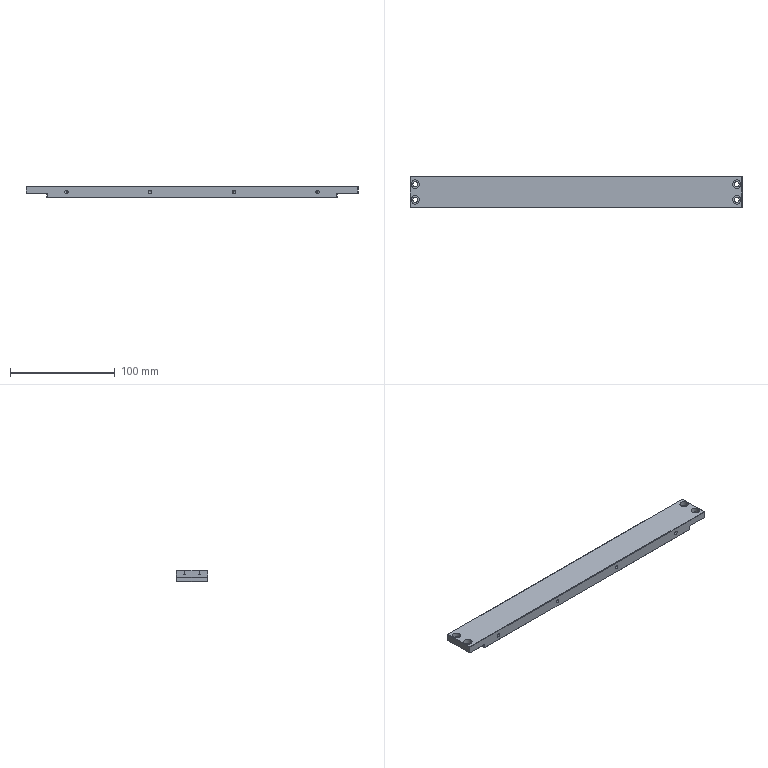Part | SolidWorks | features Chamfer 2, HoleWzd 2, Extrusion 1, ICE 1 | 1 solid | 74 faces | box 317 x 30 x 11 mm | volume 98288 mm3 | plane 42 | cylinder 24 | cone 8 | commonest cylinder face diameters 3.3 x8 4.5 x8 8 x8